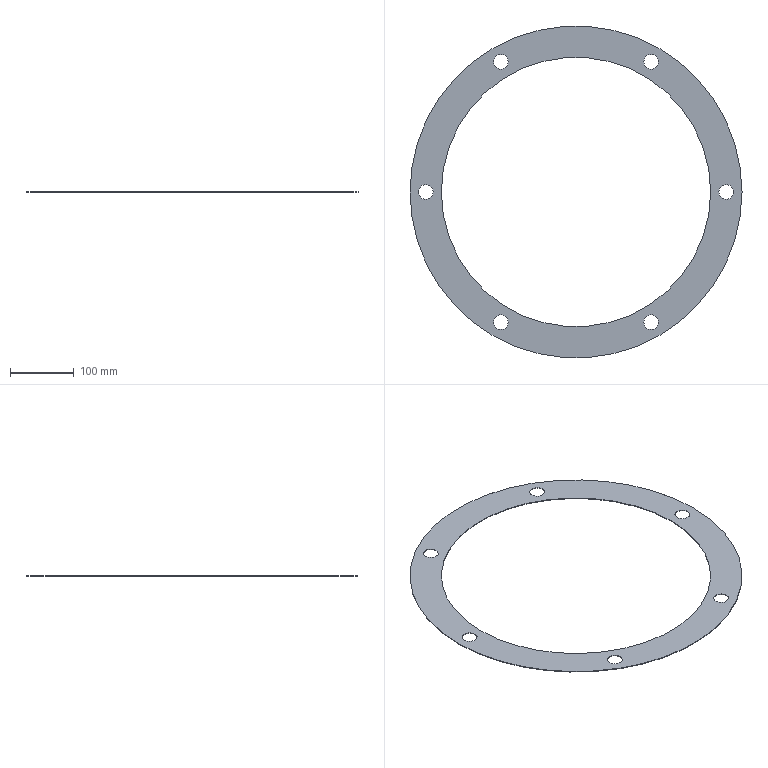Part | SolidWorks | features CirPattern 1, Extrusion 1, ICE 1 | 1 solid | 18 faces | box 519 x 519 x 1 mm | volume 69858 mm3 | cylinder 16 | plane 2 | commonest cylinder face diameters 23 x12 421 x2 519 x2
STEP:
#1=CARTESIAN_POINT('',(-106.,203.516,0.));
#2=VERTEX_POINT('',#1);
#3=CARTESIAN_POINT('',(-129.,203.516,0.));
#4=VERTEX_POINT('',#3);
#5=CARTESIAN_POINT('',(-117.5,203.516,0.));
#6=DIRECTION('',(0.,0.,-1.));
#7=DIRECTION('',(1.,0.,0.));
#8=AXIS2_PLACEMENT_3D('',#5,#6,#7);
#9=CIRCLE('',#8,11.5);
#10=EDGE_CURVE('',#2,#4,#9,.T.);
#11=ORIENTED_EDGE('',*,*,#10,.T.);
#12=CARTESIAN_POINT('',(-129.,203.516,1.));
#13=VERTEX_POINT('',#12);
#14=CARTESIAN_POINT('',(-129.,203.516,-0.001));
#15=DIRECTION('',(0.,0.,1.));
#16=VECTOR('',#15,1000.);
#17=LINE('',#14,#16);
#18=EDGE_CURVE('',#4,#13,#17,.T.);
#19=ORIENTED_EDGE('',*,*,#18,.T.);
#20=CARTESIAN_POINT('',(-106.,203.516,1.));
#21=VERTEX_POINT('',#20);
#22=CARTESIAN_POINT('',(-117.5,203.516,1.));
#23=DIRECTION('',(0.,0.,1.));
#24=DIRECTION('',(0.5,-0.866,0.));
#25=AXIS2_PLACEMENT_3D('',#22,#23,#24);
#26=CIRCLE('',#25,11.5);
#27=EDGE_CURVE('',#13,#21,#26,.T.);
#28=ORIENTED_EDGE('',*,*,#27,.T.);
#29=CARTESIAN_POINT('',(-106.,203.516,-0.001));
#30=DIRECTION('',(0.,0.,1.));
#31=VECTOR('',#30,1000.);
#32=LINE('',#29,#31);
#33=EDGE_CURVE('',#2,#21,#32,.T.);
#34=ORIENTED_EDGE('',*,*,#33,.F.);
#35=EDGE_LOOP('',(#11,#19,#28,#34));
#36=FACE_OUTER_BOUND('',#35,.T.);
#37=CARTESIAN_POINT('',(-117.5,203.516,-0.001));
#38=DIRECTION('',(0.,0.,1.));
#39=DIRECTION('',(1.,0.,0.));
#40=AXIS2_PLACEMENT_3D('',#37,#38,#39);
#41=CYLINDRICAL_SURFACE('',#40,11.5);
#42=ADVANCED_FACE('',(#36),#41,.F.);
#43=CARTESIAN_POINT('',(129.,203.516,0.));
#44=VERTEX_POINT('',#43);
#45=CARTESIAN_POINT('',(106.,203.516,0.));
#46=VERTEX_POINT('',#45);
#47=CARTESIAN_POINT('',(117.5,203.516,0.));
#48=DIRECTION('',(0.,0.,-1.));
#49=DIRECTION('',(1.,0.,0.));
#50=AXIS2_PLACEMENT_3D('',#47,#48,#49);
#51=CIRCLE('',#50,11.5);
#52=EDGE_CURVE('',#44,#46,#51,.T.);
#53=ORIENTED_EDGE('',*,*,#52,.T.);
#54=CARTESIAN_POINT('',(106.,203.516,1.));
#55=VERTEX_POINT('',#54);
#56=CARTESIAN_POINT('',(106.,203.516,-0.001));
#57=DIRECTION('',(0.,0.,1.));
#58=VECTOR('',#57,1000.);
#59=LINE('',#56,#58);
#60=EDGE_CURVE('',#46,#55,#59,.T.);
#61=ORIENTED_EDGE('',*,*,#60,.T.);
#62=CARTESIAN_POINT('',(129.,203.516,1.));
#63=VERTEX_POINT('',#62);
#64=CARTESIAN_POINT('',(117.5,203.516,1.));
#65=DIRECTION('',(0.,0.,1.));
#66=DIRECTION('',(-0.5,-0.866,0.));
#67=AXIS2_PLACEMENT_3D('',#64,#65,#66);
#68=CIRCLE('',#67,11.5);
#69=EDGE_CURVE('',#55,#63,#68,.T.);
#70=ORIENTED_EDGE('',*,*,#69,.T.);
#71=CARTESIAN_POINT('',(129.,203.516,-0.001));
#72=DIRECTION('',(0.,0.,1.));
#73=VECTOR('',#72,1000.);
#74=LINE('',#71,#73);
#75=EDGE_CURVE('',#44,#63,#74,.T.);
#76=ORIENTED_EDGE('',*,*,#75,.F.);
#77=EDGE_LOOP('',(#53,#61,#70,#76));
#78=FACE_OUTER_BOUND('',#77,.T.);
#79=CARTESIAN_POINT('',(117.5,203.516,-0.001));
#80=DIRECTION('',(0.,0.,1.));
#81=DIRECTION('',(1.,0.,0.));
#82=AXIS2_PLACEMENT_3D('',#79,#80,#81);
#83=CYLINDRICAL_SURFACE('',#82,11.5);
#84=ADVANCED_FACE('',(#78),#83,.F.);
#85=CARTESIAN_POINT('',(246.5,0.,0.));
#86=VERTEX_POINT('',#85);
#87=CARTESIAN_POINT('',(223.5,0.,0.));
#88=VERTEX_POINT('',#87);
#89=CARTESIAN_POINT('',(235.,0.,0.));
#90=DIRECTION('',(0.,0.,-1.));
#91=DIRECTION('',(1.,0.,0.));
#92=AXIS2_PLACEMENT_3D('',#89,#90,#91);
#93=CIRCLE('',#92,11.5);
#94=EDGE_CURVE('',#86,#88,#93,.T.);
#95=ORIENTED_EDGE('',*,*,#94,.T.);
#96=CARTESIAN_POINT('',(223.5,0.,1.));
#97=VERTEX_POINT('',#96);
#98=CARTESIAN_POINT('',(223.5,0.,-0.001));
#99=DIRECTION('',(0.,0.,1.));
#100=VECTOR('',#99,1000.);
#101=LINE('',#98,#100);
#102=EDGE_CURVE('',#88,#97,#101,.T.);
#103=ORIENTED_EDGE('',*,*,#102,.T.);
#104=CARTESIAN_POINT('',(246.5,0.,1.));
#105=VERTEX_POINT('',#104);
#106=CARTESIAN_POINT('',(235.,0.,1.));
#107=DIRECTION('',(0.,0.,1.));
#108=DIRECTION('',(-1.,0.,0.));
#109=AXIS2_PLACEMENT_3D('',#106,#107,#108);
#110=CIRCLE('',#109,11.5);
#111=EDGE_CURVE('',#97,#105,#110,.T.);
#112=ORIENTED_EDGE('',*,*,#111,.T.);
#113=CARTESIAN_POINT('',(246.5,0.,-0.001));
#114=DIRECTION('',(0.,0.,1.));
#115=VECTOR('',#114,1000.);
#116=LINE('',#113,#115);
#117=EDGE_CURVE('',#86,#105,#116,.T.);
#118=ORIENTED_EDGE('',*,*,#117,.F.);
#119=EDGE_LOOP('',(#95,#103,#112,#118));
#120=FACE_OUTER_BOUND('',#119,.T.);
#121=CARTESIAN_POINT('',(235.,0.,-0.001));
#122=DIRECTION('',(0.,0.,1.));
#123=DIRECTION('',(1.,0.,0.));
#124=AXIS2_PLACEMENT_3D('',#121,#122,#123);
#125=CYLINDRICAL_SURFACE('',#124,11.5);
#126=ADVANCED_FACE('',(#120),#125,.F.);
#127=CARTESIAN_POINT('',(129.,-203.516,0.));
#128=VERTEX_POINT('',#127);
#129=CARTESIAN_POINT('',(106.,-203.516,0.));
#130=VERTEX_POINT('',#129);
#131=CARTESIAN_POINT('',(117.5,-203.516,0.));
#132=DIRECTION('',(0.,0.,-1.));
#133=DIRECTION('',(1.,0.,0.));
#134=AXIS2_PLACEMENT_3D('',#131,#132,#133);
#135=CIRCLE('',#134,11.5);
#136=EDGE_CURVE('',#128,#130,#135,.T.);
#137=ORIENTED_EDGE('',*,*,#136,.T.);
#138=CARTESIAN_POINT('',(106.,-203.516,1.));
#139=VERTEX_POINT('',#138);
#140=CARTESIAN_POINT('',(106.,-203.516,-0.001));
#141=DIRECTION('',(0.,0.,1.));
#142=VECTOR('',#141,1000.);
#143=LINE('',#140,#142);
#144=EDGE_CURVE('',#130,#139,#143,.T.);
#145=ORIENTED_EDGE('',*,*,#144,.T.);
#146=CARTESIAN_POINT('',(129.,-203.516,1.));
#147=VERTEX_POINT('',#146);
#148=CARTESIAN_POINT('',(117.5,-203.516,1.));
#149=DIRECTION('',(0.,0.,1.));
#150=DIRECTION('',(-0.5,0.866,0.));
#151=AXIS2_PLACEMENT_3D('',#148,#149,#150);
#152=CIRCLE('',#151,11.5);
#153=EDGE_CURVE('',#139,#147,#152,.T.);
#154=ORIENTED_EDGE('',*,*,#153,.T.);
#155=CARTESIAN_POINT('',(129.,-203.516,-0.001));
#156=DIRECTION('',(0.,0.,1.));
#157=VECTOR('',#156,1000.);
#158=LINE('',#155,#157);
#159=EDGE_CURVE('',#128,#147,#158,.T.);
#160=ORIENTED_EDGE('',*,*,#159,.F.);
#161=EDGE_LOOP('',(#137,#145,#154,#160));
#162=FACE_OUTER_BOUND('',#161,.T.);
#163=CARTESIAN_POINT('',(117.5,-203.516,-0.001));
#164=DIRECTION('',(0.,0.,1.));
#165=DIRECTION('',(1.,0.,0.));
#166=AXIS2_PLACEMENT_3D('',#163,#164,#165);
#167=CYLINDRICAL_SURFACE('',#166,11.5);
#168=ADVANCED_FACE('',(#162),#167,.F.);
#169=CARTESIAN_POINT('',(-106.,-203.516,0.));
#170=VERTEX_POINT('',#169);
#171=CARTESIAN_POINT('',(-129.,-203.516,0.));
#172=VERTEX_POINT('',#171);
#173=CARTESIAN_POINT('',(-117.5,-203.516,0.));
#174=DIRECTION('',(0.,0.,-1.));
#175=DIRECTION('',(1.,0.,0.));
#176=AXIS2_PLACEMENT_3D('',#173,#174,#175);
#177=CIRCLE('',#176,11.5);
#178=EDGE_CURVE('',#170,#172,#177,.T.);
#179=ORIENTED_EDGE('',*,*,#178,.T.);
#180=CARTESIAN_POINT('',(-129.,-203.516,1.));
#181=VERTEX_POINT('',#180);
#182=CARTESIAN_POINT('',(-129.,-203.516,-0.001));
#183=DIRECTION('',(0.,0.,1.));
#184=VECTOR('',#183,1000.);
#185=LINE('',#182,#184);
#186=EDGE_CURVE('',#172,#181,#185,.T.);
#187=ORIENTED_EDGE('',*,*,#186,.T.);
#188=CARTESIAN_POINT('',(-106.,-203.516,1.));
#189=VERTEX_POINT('',#188);
#190=CARTESIAN_POINT('',(-117.5,-203.516,1.));
#191=DIRECTION('',(0.,0.,1.));
#192=DIRECTION('',(0.5,0.866,0.));
#193=AXIS2_PLACEMENT_3D('',#190,#191,#192);
#194=CIRCLE('',#193,11.5);
#195=EDGE_CURVE('',#181,#189,#194,.T.);
#196=ORIENTED_EDGE('',*,*,#195,.T.);
#197=CARTESIAN_POINT('',(-106.,-203.516,-0.001));
#198=DIRECTION('',(0.,0.,1.));
#199=VECTOR('',#198,1000.);
#200=LINE('',#197,#199);
#201=EDGE_CURVE('',#170,#189,#200,.T.);
#202=ORIENTED_EDGE('',*,*,#201,.F.);
#203=EDGE_LOOP('',(#179,#187,#196,#202));
#204=FACE_OUTER_BOUND('',#203,.T.);
#205=CARTESIAN_POINT('',(-117.5,-203.516,-0.001));
#206=DIRECTION('',(0.,0.,1.));
#207=DIRECTION('',(1.,0.,0.));
#208=AXIS2_PLACEMENT_3D('',#205,#206,#207);
#209=CYLINDRICAL_SURFACE('',#208,11.5);
#210=ADVANCED_FACE('',(#204),#209,.F.);
#211=CARTESIAN_POINT('',(-223.5,0.,0.));
#212=VERTEX_POINT('',#211);
#213=CARTESIAN_POINT('',(-246.5,0.,0.));
#214=VERTEX_POINT('',#213);
#215=CARTESIAN_POINT('',(-235.,0.,0.));
#216=DIRECTION('',(0.,0.,-1.));
#217=DIRECTION('',(1.,0.,0.));
#218=AXIS2_PLACEMENT_3D('',#215,#216,#217);
#219=CIRCLE('',#218,11.5);
#220=EDGE_CURVE('',#212,#214,#219,.T.);
#221=ORIENTED_EDGE('',*,*,#220,.T.);
#222=CARTESIAN_POINT('',(-246.5,0.,1.));
#223=VERTEX_POINT('',#222);
#224=CARTESIAN_POINT('',(-246.5,0.,-0.001));
#225=DIRECTION('',(0.,0.,1.));
#226=VECTOR('',#225,1000.);
#227=LINE('',#224,#226);
#228=EDGE_CURVE('',#214,#223,#227,.T.);
#229=ORIENTED_EDGE('',*,*,#228,.T.);
#230=CARTESIAN_POINT('',(-223.5,0.,1.));
#231=VERTEX_POINT('',#230);
#232=CARTESIAN_POINT('',(-235.,0.,1.));
#233=DIRECTION('',(0.,0.,1.));
#234=DIRECTION('',(1.,0.,0.));
#235=AXIS2_PLACEMENT_3D('',#232,#233,#234);
#236=CIRCLE('',#235,11.5);
#237=EDGE_CURVE('',#223,#231,#236,.T.);
#238=ORIENTED_EDGE('',*,*,#237,.T.);
#239=CARTESIAN_POINT('',(-223.5,0.,-0.001));
#240=DIRECTION('',(0.,0.,1.));
#241=VECTOR('',#240,1000.);
#242=LINE('',#239,#241);
#243=EDGE_CURVE('',#212,#231,#242,.T.);
#244=ORIENTED_EDGE('',*,*,#243,.F.);
#245=EDGE_LOOP('',(#221,#229,#238,#244));
#246=FACE_OUTER_BOUND('',#245,.T.);
#247=CARTESIAN_POINT('',(-235.,0.,-0.001));
#248=DIRECTION('',(0.,0.,1.));
#249=DIRECTION('',(1.,0.,0.));
#250=AXIS2_PLACEMENT_3D('',#247,#248,#249);
#251=CYLINDRICAL_SURFACE('',#250,11.5);
#252=ADVANCED_FACE('',(#246),#251,.F.);
#253=CARTESIAN_POINT('',(-210.5,0.,1.));
#254=VERTEX_POINT('',#253);
#255=CARTESIAN_POINT('',(210.5,0.,1.));
#256=VERTEX_POINT('',#255);
#257=CARTESIAN_POINT('',(0.,0.,1.));
#258=DIRECTION('',(0.,0.,1.));
#259=DIRECTION('',(1.,0.,0.));
#260=AXIS2_PLACEMENT_3D('',#257,#258,#259);
#261=CIRCLE('',#260,210.5);
#262=EDGE_CURVE('',#254,#256,#261,.T.);
#263=ORIENTED_EDGE('',*,*,#262,.T.);
#264=CARTESIAN_POINT('',(210.5,0.,0.));
#265=VERTEX_POINT('',#264);
#266=CARTESIAN_POINT('',(210.5,0.,1.));
#267=DIRECTION('',(0.,0.,-1.));
#268=VECTOR('',#267,1000.);
#269=LINE('',#266,#268);
#270=EDGE_CURVE('',#256,#265,#269,.T.);
#271=ORIENTED_EDGE('',*,*,#270,.T.);
#272=CARTESIAN_POINT('',(-210.5,0.,0.));
#273=VERTEX_POINT('',#272);
#274=CARTESIAN_POINT('',(0.,0.,0.));
#275=DIRECTION('',(0.,0.,1.));
#276=DIRECTION('',(1.,0.,0.));
#277=AXIS2_PLACEMENT_3D('',#274,#275,#276);
#278=CIRCLE('',#277,210.5);
#279=EDGE_CURVE('',#273,#265,#278,.T.);
#280=ORIENTED_EDGE('',*,*,#279,.F.);
#281=CARTESIAN_POINT('',(-210.5,0.,1.));
#282=DIRECTION('',(0.,0.,-1.));
#283=VECTOR('',#282,1000.);
#284=LINE('',#281,#283);
#285=EDGE_CURVE('',#254,#273,#284,.T.);
#286=ORIENTED_EDGE('',*,*,#285,.F.);
#287=EDGE_LOOP('',(#263,#271,#280,#286));
#288=FACE_OUTER_BOUND('',#287,.T.);
#289=CARTESIAN_POINT('',(0.,0.,1.));
#290=DIRECTION('',(0.,0.,-1.));
#291=DIRECTION('',(-1.,0.,0.));
#292=AXIS2_PLACEMENT_3D('',#289,#290,#291);
#293=CYLINDRICAL_SURFACE('',#292,210.5);
#294=ADVANCED_FACE('',(#288),#293,.F.);
#295=CARTESIAN_POINT('',(259.5,0.,1.));
#296=VERTEX_POINT('',#295);
#297=CARTESIAN_POINT('',(-259.5,0.,1.));
#298=VERTEX_POINT('',#297);
#299=CARTESIAN_POINT('',(0.,0.,1.));
#300=DIRECTION('',(0.,0.,1.));
#301=DIRECTION('',(1.,0.,0.));
#302=AXIS2_PLACEMENT_3D('',#299,#300,#301);
#303=CIRCLE('',#302,259.5);
#304=EDGE_CURVE('',#296,#298,#303,.T.);
#305=ORIENTED_EDGE('',*,*,#304,.F.);
#306=CARTESIAN_POINT('',(259.5,0.,0.));
#307=VERTEX_POINT('',#306);
#308=CARTESIAN_POINT('',(259.5,0.,1.));
#309=DIRECTION('',(0.,0.,-1.));
#310=VECTOR('',#309,1000.);
#311=LINE('',#308,#310);
#312=EDGE_CURVE('',#296,#307,#311,.T.);
#313=ORIENTED_EDGE('',*,*,#312,.T.);
#314=CARTESIAN_POINT('',(-259.5,0.,0.));
#315=VERTEX_POINT('',#314);
#316=CARTESIAN_POINT('',(0.,0.,0.));
#317=DIRECTION('',(0.,0.,1.));
#318=DIRECTION('',(1.,0.,0.));
#319=AXIS2_PLACEMENT_3D('',#316,#317,#318);
#320=CIRCLE('',#319,259.5);
#321=EDGE_CURVE('',#307,#315,#320,.T.);
#322=ORIENTED_EDGE('',*,*,#321,.T.);
#323=CARTESIAN_POINT('',(-259.5,0.,1.));
#324=DIRECTION('',(0.,0.,-1.));
#325=VECTOR('',#324,1000.);
#326=LINE('',#323,#325);
#327=EDGE_CURVE('',#298,#315,#326,.T.);
#328=ORIENTED_EDGE('',*,*,#327,.F.);
#329=EDGE_LOOP('',(#305,#313,#322,#328));
#330=FACE_OUTER_BOUND('',#329,.T.);
#331=CARTESIAN_POINT('',(0.,0.,1.));
#332=DIRECTION('',(0.,0.,-1.));
#333=DIRECTION('',(-1.,0.,0.));
#334=AXIS2_PLACEMENT_3D('',#331,#332,#333);
#335=CYLINDRICAL_SURFACE('',#334,259.5);
#336=ADVANCED_FACE('',(#330),#335,.T.);
#337=CARTESIAN_POINT('',(-117.5,203.516,1.));
#338=DIRECTION('',(0.,0.,1.));
#339=DIRECTION('',(0.5,-0.866,0.));
#340=AXIS2_PLACEMENT_3D('',#337,#338,#339);
#341=CIRCLE('',#340,11.5);
#342=EDGE_CURVE('',#21,#13,#341,.T.);
#343=ORIENTED_EDGE('',*,*,#342,.F.);
#344=ORIENTED_EDGE('',*,*,#27,.F.);
#345=EDGE_LOOP('',(#343,#344));
#346=FACE_BOUND('',#345,.T.);
#347=CARTESIAN_POINT('',(117.5,203.516,1.));
#348=DIRECTION('',(0.,0.,1.));
#349=DIRECTION('',(-0.5,-0.866,0.));
#350=AXIS2_PLACEMENT_3D('',#347,#348,#349);
#351=CIRCLE('',#350,11.5);
#352=EDGE_CURVE('',#63,#55,#351,.T.);
#353=ORIENTED_EDGE('',*,*,#352,.F.);
#354=ORIENTED_EDGE('',*,*,#69,.F.);
#355=EDGE_LOOP('',(#353,#354));
#356=FACE_BOUND('',#355,.T.);
#357=CARTESIAN_POINT('',(235.,0.,1.));
#358=DIRECTION('',(0.,0.,1.));
#359=DIRECTION('',(-1.,0.,0.));
#360=AXIS2_PLACEMENT_3D('',#357,#358,#359);
#361=CIRCLE('',#360,11.5);
#362=EDGE_CURVE('',#105,#97,#361,.T.);
#363=ORIENTED_EDGE('',*,*,#362,.F.);
#364=ORIENTED_EDGE('',*,*,#111,.F.);
#365=EDGE_LOOP('',(#363,#364));
#366=FACE_BOUND('',#365,.T.);
#367=CARTESIAN_POINT('',(117.5,-203.516,1.));
#368=DIRECTION('',(0.,0.,1.));
#369=DIRECTION('',(-0.5,0.866,0.));
#370=AXIS2_PLACEMENT_3D('',#367,#368,#369);
#371=CIRCLE('',#370,11.5);
#372=EDGE_CURVE('',#147,#139,#371,.T.);
#373=ORIENTED_EDGE('',*,*,#372,.F.);
#374=ORIENTED_EDGE('',*,*,#153,.F.);
#375=EDGE_LOOP('',(#373,#374));
#376=FACE_BOUND('',#375,.T.);
#377=CARTESIAN_POINT('',(-117.5,-203.516,1.));
#378=DIRECTION('',(0.,0.,1.));
#379=DIRECTION('',(0.5,0.866,0.));
#380=AXIS2_PLACEMENT_3D('',#377,#378,#379);
#381=CIRCLE('',#380,11.5);
#382=EDGE_CURVE('',#189,#181,#381,.T.);
#383=ORIENTED_EDGE('',*,*,#382,.F.);
#384=ORIENTED_EDGE('',*,*,#195,.F.);
#385=EDGE_LOOP('',(#383,#384));
#386=FACE_BOUND('',#385,.T.);
#387=CARTESIAN_POINT('',(-235.,0.,1.));
#388=DIRECTION('',(0.,0.,1.));
#389=DIRECTION('',(1.,0.,0.));
#390=AXIS2_PLACEMENT_3D('',#387,#388,#389);
#391=CIRCLE('',#390,11.5);
#392=EDGE_CURVE('',#231,#223,#391,.T.);
#393=ORIENTED_EDGE('',*,*,#392,.F.);
#394=ORIENTED_EDGE('',*,*,#237,.F.);
#395=EDGE_LOOP('',(#393,#394));
#396=FACE_BOUND('',#395,.T.);
#397=CARTESIAN_POINT('',(0.,0.,1.));
#398=DIRECTION('',(0.,0.,1.));
#399=DIRECTION('',(1.,0.,0.));
#400=AXIS2_PLACEMENT_3D('',#397,#398,#399);
#401=CIRCLE('',#400,259.5);
#402=EDGE_CURVE('',#298,#296,#401,.T.);
#403=ORIENTED_EDGE('',*,*,#402,.T.);
#404=ORIENTED_EDGE('',*,*,#304,.T.);
#405=EDGE_LOOP('',(#403,#404));
#406=FACE_OUTER_BOUND('',#405,.T.);
#407=ORIENTED_EDGE('',*,*,#262,.F.);
#408=CARTESIAN_POINT('',(0.,0.,1.));
#409=DIRECTION('',(0.,0.,1.));
#410=DIRECTION('',(1.,0.,0.));
#411=AXIS2_PLACEMENT_3D('',#408,#409,#410);
#412=CIRCLE('',#411,210.5);
#413=EDGE_CURVE('',#256,#254,#412,.T.);
#414=ORIENTED_EDGE('',*,*,#413,.F.);
#415=EDGE_LOOP('',(#407,#414));
#416=FACE_BOUND('',#415,.T.);
#417=CARTESIAN_POINT('',(0.,0.,1.));
#418=DIRECTION('',(0.,0.,1.));
#419=DIRECTION('',(1.,0.,0.));
#420=AXIS2_PLACEMENT_3D('',#417,#418,#419);
#421=PLANE('',#420);
#422=ADVANCED_FACE('',(#346,#356,#366,#376,#386,#396,#406,#416),#421,.T.);
#423=ORIENTED_EDGE('',*,*,#10,.F.);
#424=CARTESIAN_POINT('',(-117.5,203.516,0.));
#425=DIRECTION('',(0.,0.,-1.));
#426=DIRECTION('',(1.,0.,0.));
#427=AXIS2_PLACEMENT_3D('',#424,#425,#426);
#428=CIRCLE('',#427,11.5);
#429=EDGE_CURVE('',#4,#2,#428,.T.);
#430=ORIENTED_EDGE('',*,*,#429,.F.);
#431=EDGE_LOOP('',(#423,#430));
#432=FACE_BOUND('',#431,.T.);
#433=ORIENTED_EDGE('',*,*,#52,.F.);
#434=CARTESIAN_POINT('',(117.5,203.516,0.));
#435=DIRECTION('',(0.,0.,-1.));
#436=DIRECTION('',(1.,0.,0.));
#437=AXIS2_PLACEMENT_3D('',#434,#435,#436);
#438=CIRCLE('',#437,11.5);
#439=EDGE_CURVE('',#46,#44,#438,.T.);
#440=ORIENTED_EDGE('',*,*,#439,.F.);
#441=EDGE_LOOP('',(#433,#440));
#442=FACE_BOUND('',#441,.T.);
#443=ORIENTED_EDGE('',*,*,#94,.F.);
#444=CARTESIAN_POINT('',(235.,0.,0.));
#445=DIRECTION('',(0.,0.,-1.));
#446=DIRECTION('',(1.,0.,0.));
#447=AXIS2_PLACEMENT_3D('',#444,#445,#446);
#448=CIRCLE('',#447,11.5);
#449=EDGE_CURVE('',#88,#86,#448,.T.);
#450=ORIENTED_EDGE('',*,*,#449,.F.);
#451=EDGE_LOOP('',(#443,#450));
#452=FACE_BOUND('',#451,.T.);
#453=ORIENTED_EDGE('',*,*,#136,.F.);
#454=CARTESIAN_POINT('',(117.5,-203.516,0.));
#455=DIRECTION('',(0.,0.,-1.));
#456=DIRECTION('',(1.,0.,0.));
#457=AXIS2_PLACEMENT_3D('',#454,#455,#456);
#458=CIRCLE('',#457,11.5);
#459=EDGE_CURVE('',#130,#128,#458,.T.);
#460=ORIENTED_EDGE('',*,*,#459,.F.);
#461=EDGE_LOOP('',(#453,#460));
#462=FACE_BOUND('',#461,.T.);
#463=ORIENTED_EDGE('',*,*,#178,.F.);
#464=CARTESIAN_POINT('',(-117.5,-203.516,0.));
#465=DIRECTION('',(0.,0.,-1.));
#466=DIRECTION('',(1.,0.,0.));
#467=AXIS2_PLACEMENT_3D('',#464,#465,#466);
#468=CIRCLE('',#467,11.5);
#469=EDGE_CURVE('',#172,#170,#468,.T.);
#470=ORIENTED_EDGE('',*,*,#469,.F.);
#471=EDGE_LOOP('',(#463,#470));
#472=FACE_BOUND('',#471,.T.);
#473=ORIENTED_EDGE('',*,*,#220,.F.);
#474=CARTESIAN_POINT('',(-235.,0.,0.));
#475=DIRECTION('',(0.,0.,-1.));
#476=DIRECTION('',(1.,0.,0.));
#477=AXIS2_PLACEMENT_3D('',#474,#475,#476);
#478=CIRCLE('',#477,11.5);
#479=EDGE_CURVE('',#214,#212,#478,.T.);
#480=ORIENTED_EDGE('',*,*,#479,.F.);
#481=EDGE_LOOP('',(#473,#480));
#482=FACE_BOUND('',#481,.T.);
#483=CARTESIAN_POINT('',(0.,0.,0.));
#484=DIRECTION('',(0.,0.,1.));
#485=DIRECTION('',(1.,0.,0.));
#486=AXIS2_PLACEMENT_3D('',#483,#484,#485);
#487=CIRCLE('',#486,259.5);
#488=EDGE_CURVE('',#315,#307,#487,.T.);
#489=ORIENTED_EDGE('',*,*,#488,.F.);
#490=ORIENTED_EDGE('',*,*,#321,.F.);
#491=EDGE_LOOP('',(#489,#490));
#492=FACE_OUTER_BOUND('',#491,.T.);
#493=ORIENTED_EDGE('',*,*,#279,.T.);
#494=CARTESIAN_POINT('',(0.,0.,0.));
#495=DIRECTION('',(0.,0.,1.));
#496=DIRECTION('',(1.,0.,0.));
#497=AXIS2_PLACEMENT_3D('',#494,#495,#496);
#498=CIRCLE('',#497,210.5);
#499=EDGE_CURVE('',#265,#273,#498,.T.);
#500=ORIENTED_EDGE('',*,*,#499,.T.);
#501=EDGE_LOOP('',(#493,#500));
#502=FACE_BOUND('',#501,.T.);
#503=CARTESIAN_POINT('',(0.,0.,0.));
#504=DIRECTION('',(0.,0.,1.));
#505=DIRECTION('',(1.,0.,0.));
#506=AXIS2_PLACEMENT_3D('',#503,#504,#505);
#507=PLANE('',#506);
#508=ADVANCED_FACE('',(#432,#442,#452,#462,#472,#482,#492,#502),#507,.F.);
#509=ORIENTED_EDGE('',*,*,#312,.F.);
#510=ORIENTED_EDGE('',*,*,#402,.F.);
#511=ORIENTED_EDGE('',*,*,#327,.T.);
#512=ORIENTED_EDGE('',*,*,#488,.T.);
#513=EDGE_LOOP('',(#509,#510,#511,#512));
#514=FACE_OUTER_BOUND('',#513,.T.);
#515=CARTESIAN_POINT('',(0.,0.,1.));
#516=DIRECTION('',(0.,0.,-1.));
#517=DIRECTION('',(-1.,0.,0.));
#518=AXIS2_PLACEMENT_3D('',#515,#516,#517);
#519=CYLINDRICAL_SURFACE('',#518,259.5);
#520=ADVANCED_FACE('',(#514),#519,.T.);
#521=ORIENTED_EDGE('',*,*,#270,.F.);
#522=ORIENTED_EDGE('',*,*,#413,.T.);
#523=ORIENTED_EDGE('',*,*,#285,.T.);
#524=ORIENTED_EDGE('',*,*,#499,.F.);
#525=EDGE_LOOP('',(#521,#522,#523,#524));
#526=FACE_OUTER_BOUND('',#525,.T.);
#527=CARTESIAN_POINT('',(0.,0.,1.));
#528=DIRECTION('',(0.,0.,-1.));
#529=DIRECTION('',(-1.,0.,0.));
#530=AXIS2_PLACEMENT_3D('',#527,#528,#529);
#531=CYLINDRICAL_SURFACE('',#530,210.5);
#532=ADVANCED_FACE('',(#526),#531,.F.);
#533=ORIENTED_EDGE('',*,*,#228,.F.);
#534=ORIENTED_EDGE('',*,*,#479,.T.);
#535=ORIENTED_EDGE('',*,*,#243,.T.);
#536=ORIENTED_EDGE('',*,*,#392,.T.);
#537=EDGE_LOOP('',(#533,#534,#535,#536));
#538=FACE_OUTER_BOUND('',#537,.T.);
#539=CARTESIAN_POINT('',(-235.,0.,-0.001));
#540=DIRECTION('',(0.,0.,1.));
#541=DIRECTION('',(1.,0.,0.));
#542=AXIS2_PLACEMENT_3D('',#539,#540,#541);
#543=CYLINDRICAL_SURFACE('',#542,11.5);
#544=ADVANCED_FACE('',(#538),#543,.F.);
#545=ORIENTED_EDGE('',*,*,#186,.F.);
#546=ORIENTED_EDGE('',*,*,#469,.T.);
#547=ORIENTED_EDGE('',*,*,#201,.T.);
#548=ORIENTED_EDGE('',*,*,#382,.T.);
#549=EDGE_LOOP('',(#545,#546,#547,#548));
#550=FACE_OUTER_BOUND('',#549,.T.);
#551=CARTESIAN_POINT('',(-117.5,-203.516,-0.001));
#552=DIRECTION('',(0.,0.,1.));
#553=DIRECTION('',(1.,0.,0.));
#554=AXIS2_PLACEMENT_3D('',#551,#552,#553);
#555=CYLINDRICAL_SURFACE('',#554,11.5);
#556=ADVANCED_FACE('',(#550),#555,.F.);
#557=ORIENTED_EDGE('',*,*,#144,.F.);
#558=ORIENTED_EDGE('',*,*,#459,.T.);
#559=ORIENTED_EDGE('',*,*,#159,.T.);
#560=ORIENTED_EDGE('',*,*,#372,.T.);
#561=EDGE_LOOP('',(#557,#558,#559,#560));
#562=FACE_OUTER_BOUND('',#561,.T.);
#563=CARTESIAN_POINT('',(117.5,-203.516,-0.001));
#564=DIRECTION('',(0.,0.,1.));
#565=DIRECTION('',(1.,0.,0.));
#566=AXIS2_PLACEMENT_3D('',#563,#564,#565);
#567=CYLINDRICAL_SURFACE('',#566,11.5);
#568=ADVANCED_FACE('',(#562),#567,.F.);
#569=ORIENTED_EDGE('',*,*,#102,.F.);
#570=ORIENTED_EDGE('',*,*,#449,.T.);
#571=ORIENTED_EDGE('',*,*,#117,.T.);
#572=ORIENTED_EDGE('',*,*,#362,.T.);
#573=EDGE_LOOP('',(#569,#570,#571,#572));
#574=FACE_OUTER_BOUND('',#573,.T.);
#575=CARTESIAN_POINT('',(235.,0.,-0.001));
#576=DIRECTION('',(0.,0.,1.));
#577=DIRECTION('',(1.,0.,0.));
#578=AXIS2_PLACEMENT_3D('',#575,#576,#577);
#579=CYLINDRICAL_SURFACE('',#578,11.5);
#580=ADVANCED_FACE('',(#574),#579,.F.);
#581=ORIENTED_EDGE('',*,*,#60,.F.);
#582=ORIENTED_EDGE('',*,*,#439,.T.);
#583=ORIENTED_EDGE('',*,*,#75,.T.);
#584=ORIENTED_EDGE('',*,*,#352,.T.);
#585=EDGE_LOOP('',(#581,#582,#583,#584));
#586=FACE_OUTER_BOUND('',#585,.T.);
#587=CARTESIAN_POINT('',(117.5,203.516,-0.001));
#588=DIRECTION('',(0.,0.,1.));
#589=DIRECTION('',(1.,0.,0.));
#590=AXIS2_PLACEMENT_3D('',#587,#588,#589);
#591=CYLINDRICAL_SURFACE('',#590,11.5);
#592=ADVANCED_FACE('',(#586),#591,.F.);
#593=ORIENTED_EDGE('',*,*,#18,.F.);
#594=ORIENTED_EDGE('',*,*,#429,.T.);
#595=ORIENTED_EDGE('',*,*,#33,.T.);
#596=ORIENTED_EDGE('',*,*,#342,.T.);
#597=EDGE_LOOP('',(#593,#594,#595,#596));
#598=FACE_OUTER_BOUND('',#597,.T.);
#599=CARTESIAN_POINT('',(-117.5,203.516,-0.001));
#600=DIRECTION('',(0.,0.,1.));
#601=DIRECTION('',(1.,0.,0.));
#602=AXIS2_PLACEMENT_3D('',#599,#600,#601);
#603=CYLINDRICAL_SURFACE('',#602,11.5);
#604=ADVANCED_FACE('',(#598),#603,.F.);
#605=CLOSED_SHELL('',(#42,#84,#126,#168,#210,#252,#294,#336,#422,#508,#520,#532,#544,#556,#568,#580,#592,#604));
#606=MANIFOLD_SOLID_BREP('',#605);
#607=CARTESIAN_POINT('',(0.,0.,0.));
#608=DIRECTION('',(0.,0.,1.));
#609=DIRECTION('',(1.,0.,0.));
#610=AXIS2_PLACEMENT_3D('',#607,#608,#609);
#611=(LENGTH_UNIT()NAMED_UNIT(*)SI_UNIT(.MILLI.,.METRE.));
#612=UNCERTAINTY_MEASURE_WITH_UNIT(LENGTH_MEASURE(0.00001),#611,'','');
#613=(NAMED_UNIT(*)PLANE_ANGLE_UNIT()SI_UNIT($,.RADIAN.));
#614=(NAMED_UNIT(*)SI_UNIT($,.STERADIAN.)SOLID_ANGLE_UNIT());
#615=(GEOMETRIC_REPRESENTATION_CONTEXT(3)GLOBAL_UNCERTAINTY_ASSIGNED_CONTEXT((#612))GLOBAL_UNIT_ASSIGNED_CONTEXT((#611,#613,#614))REPRESENTATION_CONTEXT('',''));
#616=ADVANCED_BREP_SHAPE_REPRESENTATION('',(#606,#610),#615);